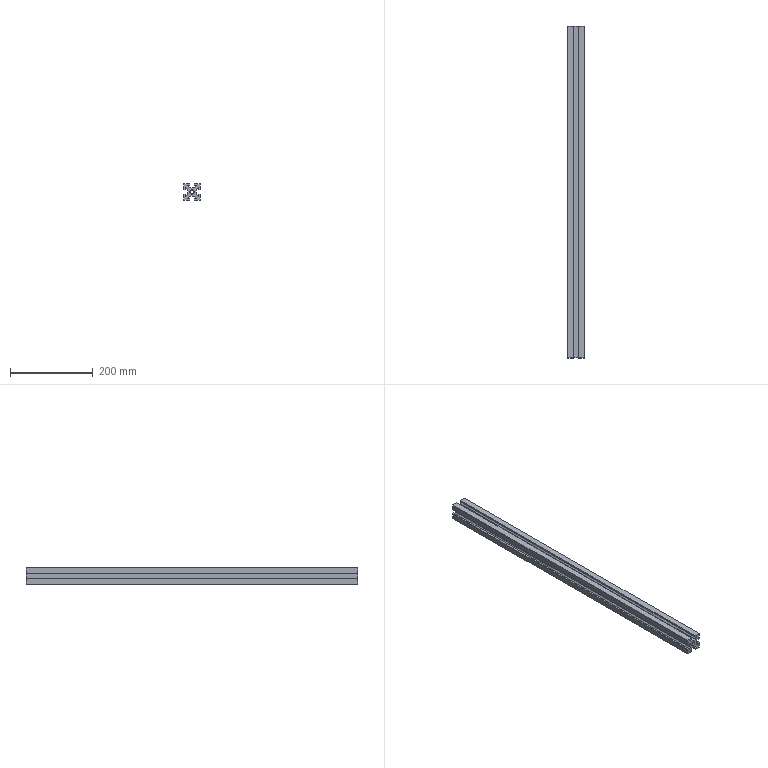Part | SolidWorks | features Extrusion 1 | 1 solid | 40 faces | box 40 x 800 x 40 mm | volume 727286 mm3 | plane 38 | cylinder 2 | commonest cylinder face diameters 10 x2
STEP:
#1=CARTESIAN_POINT('',(0.,800.,-5.));
#2=VERTEX_POINT('',#1);
#3=CARTESIAN_POINT('',(0.,800.,5.));
#4=VERTEX_POINT('',#3);
#5=CARTESIAN_POINT('',(0.,800.,0.));
#6=DIRECTION('',(0.,1.,0.));
#7=DIRECTION('',(0.,0.,1.));
#8=AXIS2_PLACEMENT_3D('',#5,#6,#7);
#9=CIRCLE('',#8,5.);
#10=EDGE_CURVE('',#2,#4,#9,.T.);
#11=ORIENTED_EDGE('',*,*,#10,.T.);
#12=CARTESIAN_POINT('',(0.,0.,5.));
#13=VERTEX_POINT('',#12);
#14=CARTESIAN_POINT('',(0.,800.,5.));
#15=DIRECTION('',(0.,-1.,0.));
#16=VECTOR('',#15,1000.);
#17=LINE('',#14,#16);
#18=EDGE_CURVE('',#4,#13,#17,.T.);
#19=ORIENTED_EDGE('',*,*,#18,.T.);
#20=CARTESIAN_POINT('',(0.,0.,-5.));
#21=VERTEX_POINT('',#20);
#22=CARTESIAN_POINT('',(0.,0.,0.));
#23=DIRECTION('',(0.,1.,0.));
#24=DIRECTION('',(0.,0.,1.));
#25=AXIS2_PLACEMENT_3D('',#22,#23,#24);
#26=CIRCLE('',#25,5.);
#27=EDGE_CURVE('',#21,#13,#26,.T.);
#28=ORIENTED_EDGE('',*,*,#27,.F.);
#29=CARTESIAN_POINT('',(0.,800.,-5.));
#30=DIRECTION('',(0.,-1.,0.));
#31=VECTOR('',#30,1000.);
#32=LINE('',#29,#31);
#33=EDGE_CURVE('',#2,#21,#32,.T.);
#34=ORIENTED_EDGE('',*,*,#33,.F.);
#35=EDGE_LOOP('',(#11,#19,#28,#34));
#36=FACE_OUTER_BOUND('',#35,.T.);
#37=CARTESIAN_POINT('',(0.,800.,0.));
#38=DIRECTION('',(0.,-1.,0.));
#39=DIRECTION('',(0.,0.,-1.));
#40=AXIS2_PLACEMENT_3D('',#37,#38,#39);
#41=CYLINDRICAL_SURFACE('',#40,5.);
#42=ADVANCED_FACE('',(#36),#41,.F.);
#43=CARTESIAN_POINT('',(6.,800.,20.));
#44=VERTEX_POINT('',#43);
#45=CARTESIAN_POINT('',(20.,800.,20.));
#46=VERTEX_POINT('',#45);
#47=CARTESIAN_POINT('',(6.,800.,20.));
#48=DIRECTION('',(1.,0.,0.));
#49=VECTOR('',#48,1000.);
#50=LINE('',#47,#49);
#51=EDGE_CURVE('',#44,#46,#50,.T.);
#52=ORIENTED_EDGE('',*,*,#51,.T.);
#53=CARTESIAN_POINT('',(20.,800.,6.));
#54=VERTEX_POINT('',#53);
#55=CARTESIAN_POINT('',(20.,800.,6.));
#56=DIRECTION('',(0.,0.,-1.));
#57=VECTOR('',#56,1000.);
#58=LINE('',#55,#57);
#59=EDGE_CURVE('',#46,#54,#58,.T.);
#60=ORIENTED_EDGE('',*,*,#59,.T.);
#61=CARTESIAN_POINT('',(16.,800.,6.));
#62=VERTEX_POINT('',#61);
#63=CARTESIAN_POINT('',(16.,800.,6.));
#64=DIRECTION('',(-1.,0.,0.));
#65=VECTOR('',#64,1000.);
#66=LINE('',#63,#65);
#67=EDGE_CURVE('',#54,#62,#66,.T.);
#68=ORIENTED_EDGE('',*,*,#67,.T.);
#69=CARTESIAN_POINT('',(16.,800.,11.757));
#70=VERTEX_POINT('',#69);
#71=CARTESIAN_POINT('',(16.,800.,11.757));
#72=DIRECTION('',(0.,0.,1.));
#73=VECTOR('',#72,1000.);
#74=LINE('',#71,#73);
#75=EDGE_CURVE('',#62,#70,#74,.T.);
#76=ORIENTED_EDGE('',*,*,#75,.T.);
#77=CARTESIAN_POINT('',(10.,800.,5.757));
#78=VERTEX_POINT('',#77);
#79=CARTESIAN_POINT('',(10.,800.,5.757));
#80=DIRECTION('',(-0.7071,0.,-0.7071));
#81=VECTOR('',#80,1000.);
#82=LINE('',#79,#81);
#83=EDGE_CURVE('',#70,#78,#82,.T.);
#84=ORIENTED_EDGE('',*,*,#83,.T.);
#85=CARTESIAN_POINT('',(10.,800.,-5.757));
#86=VERTEX_POINT('',#85);
#87=CARTESIAN_POINT('',(10.,800.,5.757));
#88=DIRECTION('',(0.,0.,-1.));
#89=VECTOR('',#88,1000.);
#90=LINE('',#87,#89);
#91=EDGE_CURVE('',#78,#86,#90,.T.);
#92=ORIENTED_EDGE('',*,*,#91,.T.);
#93=CARTESIAN_POINT('',(16.,800.,-11.757));
#94=VERTEX_POINT('',#93);
#95=CARTESIAN_POINT('',(16.,800.,-11.757));
#96=DIRECTION('',(0.7071,0.,-0.7071));
#97=VECTOR('',#96,1000.);
#98=LINE('',#95,#97);
#99=EDGE_CURVE('',#86,#94,#98,.T.);
#100=ORIENTED_EDGE('',*,*,#99,.T.);
#101=CARTESIAN_POINT('',(16.,800.,-6.));
#102=VERTEX_POINT('',#101);
#103=CARTESIAN_POINT('',(16.,800.,-6.));
#104=DIRECTION('',(0.,0.,1.));
#105=VECTOR('',#104,1000.);
#106=LINE('',#103,#105);
#107=EDGE_CURVE('',#94,#102,#106,.T.);
#108=ORIENTED_EDGE('',*,*,#107,.T.);
#109=CARTESIAN_POINT('',(20.,800.,-6.));
#110=VERTEX_POINT('',#109);
#111=CARTESIAN_POINT('',(20.,800.,-6.));
#112=DIRECTION('',(1.,0.,0.));
#113=VECTOR('',#112,1000.);
#114=LINE('',#111,#113);
#115=EDGE_CURVE('',#102,#110,#114,.T.);
#116=ORIENTED_EDGE('',*,*,#115,.T.);
#117=CARTESIAN_POINT('',(20.,800.,-20.));
#118=VERTEX_POINT('',#117);
#119=CARTESIAN_POINT('',(20.,800.,-20.));
#120=DIRECTION('',(0.,0.,-1.));
#121=VECTOR('',#120,1000.);
#122=LINE('',#119,#121);
#123=EDGE_CURVE('',#110,#118,#122,.T.);
#124=ORIENTED_EDGE('',*,*,#123,.T.);
#125=CARTESIAN_POINT('',(6.,800.,-20.));
#126=VERTEX_POINT('',#125);
#127=CARTESIAN_POINT('',(6.,800.,-20.));
#128=DIRECTION('',(-1.,0.,0.));
#129=VECTOR('',#128,1000.);
#130=LINE('',#127,#129);
#131=EDGE_CURVE('',#118,#126,#130,.T.);
#132=ORIENTED_EDGE('',*,*,#131,.T.);
#133=CARTESIAN_POINT('',(6.,800.,-16.));
#134=VERTEX_POINT('',#133);
#135=CARTESIAN_POINT('',(6.,800.,-16.));
#136=DIRECTION('',(0.,0.,1.));
#137=VECTOR('',#136,1000.);
#138=LINE('',#135,#137);
#139=EDGE_CURVE('',#126,#134,#138,.T.);
#140=ORIENTED_EDGE('',*,*,#139,.T.);
#141=CARTESIAN_POINT('',(11.757,800.,-16.));
#142=VERTEX_POINT('',#141);
#143=CARTESIAN_POINT('',(11.757,800.,-16.));
#144=DIRECTION('',(1.,0.,0.));
#145=VECTOR('',#144,1000.);
#146=LINE('',#143,#145);
#147=EDGE_CURVE('',#134,#142,#146,.T.);
#148=ORIENTED_EDGE('',*,*,#147,.T.);
#149=CARTESIAN_POINT('',(5.757,800.,-10.));
#150=VERTEX_POINT('',#149);
#151=CARTESIAN_POINT('',(5.757,800.,-10.));
#152=DIRECTION('',(-0.7071,0.,0.7071));
#153=VECTOR('',#152,1000.);
#154=LINE('',#151,#153);
#155=EDGE_CURVE('',#142,#150,#154,.T.);
#156=ORIENTED_EDGE('',*,*,#155,.T.);
#157=CARTESIAN_POINT('',(-5.757,800.,-10.));
#158=VERTEX_POINT('',#157);
#159=CARTESIAN_POINT('',(-5.757,800.,-10.));
#160=DIRECTION('',(-1.,0.,0.));
#161=VECTOR('',#160,1000.);
#162=LINE('',#159,#161);
#163=EDGE_CURVE('',#150,#158,#162,.T.);
#164=ORIENTED_EDGE('',*,*,#163,.T.);
#165=CARTESIAN_POINT('',(-11.757,800.,-16.));
#166=VERTEX_POINT('',#165);
#167=CARTESIAN_POINT('',(-11.757,800.,-16.));
#168=DIRECTION('',(-0.7071,0.,-0.7071));
#169=VECTOR('',#168,1000.);
#170=LINE('',#167,#169);
#171=EDGE_CURVE('',#158,#166,#170,.T.);
#172=ORIENTED_EDGE('',*,*,#171,.T.);
#173=CARTESIAN_POINT('',(-6.,800.,-16.));
#174=VERTEX_POINT('',#173);
#175=CARTESIAN_POINT('',(-6.,800.,-16.));
#176=DIRECTION('',(1.,0.,0.));
#177=VECTOR('',#176,1000.);
#178=LINE('',#175,#177);
#179=EDGE_CURVE('',#166,#174,#178,.T.);
#180=ORIENTED_EDGE('',*,*,#179,.T.);
#181=CARTESIAN_POINT('',(-6.,800.,-20.));
#182=VERTEX_POINT('',#181);
#183=CARTESIAN_POINT('',(-6.,800.,-20.));
#184=DIRECTION('',(0.,0.,-1.));
#185=VECTOR('',#184,1000.);
#186=LINE('',#183,#185);
#187=EDGE_CURVE('',#174,#182,#186,.T.);
#188=ORIENTED_EDGE('',*,*,#187,.T.);
#189=CARTESIAN_POINT('',(-20.,800.,-20.));
#190=VERTEX_POINT('',#189);
#191=CARTESIAN_POINT('',(-20.,800.,-20.));
#192=DIRECTION('',(-1.,0.,0.));
#193=VECTOR('',#192,1000.);
#194=LINE('',#191,#193);
#195=EDGE_CURVE('',#182,#190,#194,.T.);
#196=ORIENTED_EDGE('',*,*,#195,.T.);
#197=CARTESIAN_POINT('',(-20.,800.,-6.));
#198=VERTEX_POINT('',#197);
#199=CARTESIAN_POINT('',(-20.,800.,-20.));
#200=DIRECTION('',(0.,0.,1.));
#201=VECTOR('',#200,1000.);
#202=LINE('',#199,#201);
#203=EDGE_CURVE('',#190,#198,#202,.T.);
#204=ORIENTED_EDGE('',*,*,#203,.T.);
#205=CARTESIAN_POINT('',(-16.,800.,-6.));
#206=VERTEX_POINT('',#205);
#207=CARTESIAN_POINT('',(-16.,800.,-6.));
#208=DIRECTION('',(1.,0.,0.));
#209=VECTOR('',#208,1000.);
#210=LINE('',#207,#209);
#211=EDGE_CURVE('',#198,#206,#210,.T.);
#212=ORIENTED_EDGE('',*,*,#211,.T.);
#213=CARTESIAN_POINT('',(-16.,800.,-11.757));
#214=VERTEX_POINT('',#213);
#215=CARTESIAN_POINT('',(-16.,800.,-11.757));
#216=DIRECTION('',(0.,0.,-1.));
#217=VECTOR('',#216,1000.);
#218=LINE('',#215,#217);
#219=EDGE_CURVE('',#206,#214,#218,.T.);
#220=ORIENTED_EDGE('',*,*,#219,.T.);
#221=CARTESIAN_POINT('',(-10.,800.,-5.757));
#222=VERTEX_POINT('',#221);
#223=CARTESIAN_POINT('',(-10.,800.,-5.757));
#224=DIRECTION('',(0.7071,0.,0.7071));
#225=VECTOR('',#224,1000.);
#226=LINE('',#223,#225);
#227=EDGE_CURVE('',#214,#222,#226,.T.);
#228=ORIENTED_EDGE('',*,*,#227,.T.);
#229=CARTESIAN_POINT('',(-10.,800.,5.757));
#230=VERTEX_POINT('',#229);
#231=CARTESIAN_POINT('',(-10.,800.,5.757));
#232=DIRECTION('',(0.,0.,1.));
#233=VECTOR('',#232,1000.);
#234=LINE('',#231,#233);
#235=EDGE_CURVE('',#222,#230,#234,.T.);
#236=ORIENTED_EDGE('',*,*,#235,.T.);
#237=CARTESIAN_POINT('',(-16.,800.,11.757));
#238=VERTEX_POINT('',#237);
#239=CARTESIAN_POINT('',(-16.,800.,11.757));
#240=DIRECTION('',(-0.7071,0.,0.7071));
#241=VECTOR('',#240,1000.);
#242=LINE('',#239,#241);
#243=EDGE_CURVE('',#230,#238,#242,.T.);
#244=ORIENTED_EDGE('',*,*,#243,.T.);
#245=CARTESIAN_POINT('',(-16.,800.,6.));
#246=VERTEX_POINT('',#245);
#247=CARTESIAN_POINT('',(-16.,800.,6.));
#248=DIRECTION('',(0.,0.,-1.));
#249=VECTOR('',#248,1000.);
#250=LINE('',#247,#249);
#251=EDGE_CURVE('',#238,#246,#250,.T.);
#252=ORIENTED_EDGE('',*,*,#251,.T.);
#253=CARTESIAN_POINT('',(-20.,800.,6.));
#254=VERTEX_POINT('',#253);
#255=CARTESIAN_POINT('',(-20.,800.,6.));
#256=DIRECTION('',(-1.,0.,0.));
#257=VECTOR('',#256,1000.);
#258=LINE('',#255,#257);
#259=EDGE_CURVE('',#246,#254,#258,.T.);
#260=ORIENTED_EDGE('',*,*,#259,.T.);
#261=CARTESIAN_POINT('',(-20.,800.,20.));
#262=VERTEX_POINT('',#261);
#263=CARTESIAN_POINT('',(-20.,800.,6.));
#264=DIRECTION('',(0.,0.,1.));
#265=VECTOR('',#264,1000.);
#266=LINE('',#263,#265);
#267=EDGE_CURVE('',#254,#262,#266,.T.);
#268=ORIENTED_EDGE('',*,*,#267,.T.);
#269=CARTESIAN_POINT('',(-6.,800.,20.));
#270=VERTEX_POINT('',#269);
#271=CARTESIAN_POINT('',(-20.,800.,20.));
#272=DIRECTION('',(1.,0.,0.));
#273=VECTOR('',#272,1000.);
#274=LINE('',#271,#273);
#275=EDGE_CURVE('',#262,#270,#274,.T.);
#276=ORIENTED_EDGE('',*,*,#275,.T.);
#277=CARTESIAN_POINT('',(-6.,800.,16.));
#278=VERTEX_POINT('',#277);
#279=CARTESIAN_POINT('',(-6.,800.,16.));
#280=DIRECTION('',(0.,0.,-1.));
#281=VECTOR('',#280,1000.);
#282=LINE('',#279,#281);
#283=EDGE_CURVE('',#270,#278,#282,.T.);
#284=ORIENTED_EDGE('',*,*,#283,.T.);
#285=CARTESIAN_POINT('',(-11.757,800.,16.));
#286=VERTEX_POINT('',#285);
#287=CARTESIAN_POINT('',(-11.757,800.,16.));
#288=DIRECTION('',(-1.,0.,0.));
#289=VECTOR('',#288,1000.);
#290=LINE('',#287,#289);
#291=EDGE_CURVE('',#278,#286,#290,.T.);
#292=ORIENTED_EDGE('',*,*,#291,.T.);
#293=CARTESIAN_POINT('',(-5.757,800.,10.));
#294=VERTEX_POINT('',#293);
#295=CARTESIAN_POINT('',(-5.757,800.,10.));
#296=DIRECTION('',(0.7071,0.,-0.7071));
#297=VECTOR('',#296,1000.);
#298=LINE('',#295,#297);
#299=EDGE_CURVE('',#286,#294,#298,.T.);
#300=ORIENTED_EDGE('',*,*,#299,.T.);
#301=CARTESIAN_POINT('',(5.757,800.,10.));
#302=VERTEX_POINT('',#301);
#303=CARTESIAN_POINT('',(-5.757,800.,10.));
#304=DIRECTION('',(1.,0.,0.));
#305=VECTOR('',#304,1000.);
#306=LINE('',#303,#305);
#307=EDGE_CURVE('',#294,#302,#306,.T.);
#308=ORIENTED_EDGE('',*,*,#307,.T.);
#309=CARTESIAN_POINT('',(11.757,800.,16.));
#310=VERTEX_POINT('',#309);
#311=CARTESIAN_POINT('',(11.757,800.,16.));
#312=DIRECTION('',(0.7071,0.,0.7071));
#313=VECTOR('',#312,1000.);
#314=LINE('',#311,#313);
#315=EDGE_CURVE('',#302,#310,#314,.T.);
#316=ORIENTED_EDGE('',*,*,#315,.T.);
#317=CARTESIAN_POINT('',(6.,800.,16.));
#318=VERTEX_POINT('',#317);
#319=CARTESIAN_POINT('',(6.,800.,16.));
#320=DIRECTION('',(-1.,0.,0.));
#321=VECTOR('',#320,1000.);
#322=LINE('',#319,#321);
#323=EDGE_CURVE('',#310,#318,#322,.T.);
#324=ORIENTED_EDGE('',*,*,#323,.T.);
#325=CARTESIAN_POINT('',(6.,800.,20.));
#326=DIRECTION('',(0.,0.,1.));
#327=VECTOR('',#326,1000.);
#328=LINE('',#325,#327);
#329=EDGE_CURVE('',#318,#44,#328,.T.);
#330=ORIENTED_EDGE('',*,*,#329,.T.);
#331=EDGE_LOOP('',(#52,#60,#68,#76,#84,#92,#100,#108,#116,#124,#132,#140,#148,#156,#164,#172,#180,#188,#196,#204,#212,#220,#228,#236,#244,#252,#260,#268,#276,#284,#292,#300,#308,#316,#324,#330));
#332=FACE_OUTER_BOUND('',#331,.T.);
#333=ORIENTED_EDGE('',*,*,#10,.F.);
#334=CARTESIAN_POINT('',(0.,800.,0.));
#335=DIRECTION('',(0.,1.,0.));
#336=DIRECTION('',(0.,0.,1.));
#337=AXIS2_PLACEMENT_3D('',#334,#335,#336);
#338=CIRCLE('',#337,5.);
#339=EDGE_CURVE('',#4,#2,#338,.T.);
#340=ORIENTED_EDGE('',*,*,#339,.F.);
#341=EDGE_LOOP('',(#333,#340));
#342=FACE_BOUND('',#341,.T.);
#343=CARTESIAN_POINT('',(0.,800.,0.));
#344=DIRECTION('',(0.,-1.,0.));
#345=DIRECTION('',(0.,0.,-1.));
#346=AXIS2_PLACEMENT_3D('',#343,#344,#345);
#347=PLANE('',#346);
#348=ADVANCED_FACE('',(#332,#342),#347,.F.);
#349=CARTESIAN_POINT('',(6.,0.,20.));
#350=VERTEX_POINT('',#349);
#351=CARTESIAN_POINT('',(20.,0.,20.));
#352=VERTEX_POINT('',#351);
#353=CARTESIAN_POINT('',(6.,0.,20.));
#354=DIRECTION('',(1.,0.,0.));
#355=VECTOR('',#354,1000.);
#356=LINE('',#353,#355);
#357=EDGE_CURVE('',#350,#352,#356,.T.);
#358=ORIENTED_EDGE('',*,*,#357,.F.);
#359=CARTESIAN_POINT('',(6.,0.,16.));
#360=VERTEX_POINT('',#359);
#361=CARTESIAN_POINT('',(6.,0.,20.));
#362=DIRECTION('',(0.,0.,1.));
#363=VECTOR('',#362,1000.);
#364=LINE('',#361,#363);
#365=EDGE_CURVE('',#360,#350,#364,.T.);
#366=ORIENTED_EDGE('',*,*,#365,.F.);
#367=CARTESIAN_POINT('',(11.757,0.,16.));
#368=VERTEX_POINT('',#367);
#369=CARTESIAN_POINT('',(6.,0.,16.));
#370=DIRECTION('',(-1.,0.,0.));
#371=VECTOR('',#370,1000.);
#372=LINE('',#369,#371);
#373=EDGE_CURVE('',#368,#360,#372,.T.);
#374=ORIENTED_EDGE('',*,*,#373,.F.);
#375=CARTESIAN_POINT('',(5.757,0.,10.));
#376=VERTEX_POINT('',#375);
#377=CARTESIAN_POINT('',(11.757,0.,16.));
#378=DIRECTION('',(0.7071,0.,0.7071));
#379=VECTOR('',#378,1000.);
#380=LINE('',#377,#379);
#381=EDGE_CURVE('',#376,#368,#380,.T.);
#382=ORIENTED_EDGE('',*,*,#381,.F.);
#383=CARTESIAN_POINT('',(-5.757,0.,10.));
#384=VERTEX_POINT('',#383);
#385=CARTESIAN_POINT('',(-5.757,0.,10.));
#386=DIRECTION('',(1.,0.,0.));
#387=VECTOR('',#386,1000.);
#388=LINE('',#385,#387);
#389=EDGE_CURVE('',#384,#376,#388,.T.);
#390=ORIENTED_EDGE('',*,*,#389,.F.);
#391=CARTESIAN_POINT('',(-11.757,0.,16.));
#392=VERTEX_POINT('',#391);
#393=CARTESIAN_POINT('',(-5.757,0.,10.));
#394=DIRECTION('',(0.7071,0.,-0.7071));
#395=VECTOR('',#394,1000.);
#396=LINE('',#393,#395);
#397=EDGE_CURVE('',#392,#384,#396,.T.);
#398=ORIENTED_EDGE('',*,*,#397,.F.);
#399=CARTESIAN_POINT('',(-6.,0.,16.));
#400=VERTEX_POINT('',#399);
#401=CARTESIAN_POINT('',(-11.757,0.,16.));
#402=DIRECTION('',(-1.,0.,0.));
#403=VECTOR('',#402,1000.);
#404=LINE('',#401,#403);
#405=EDGE_CURVE('',#400,#392,#404,.T.);
#406=ORIENTED_EDGE('',*,*,#405,.F.);
#407=CARTESIAN_POINT('',(-6.,0.,20.));
#408=VERTEX_POINT('',#407);
#409=CARTESIAN_POINT('',(-6.,0.,16.));
#410=DIRECTION('',(0.,0.,-1.));
#411=VECTOR('',#410,1000.);
#412=LINE('',#409,#411);
#413=EDGE_CURVE('',#408,#400,#412,.T.);
#414=ORIENTED_EDGE('',*,*,#413,.F.);
#415=CARTESIAN_POINT('',(-20.,0.,20.));
#416=VERTEX_POINT('',#415);
#417=CARTESIAN_POINT('',(-20.,0.,20.));
#418=DIRECTION('',(1.,0.,0.));
#419=VECTOR('',#418,1000.);
#420=LINE('',#417,#419);
#421=EDGE_CURVE('',#416,#408,#420,.T.);
#422=ORIENTED_EDGE('',*,*,#421,.F.);
#423=CARTESIAN_POINT('',(-20.,0.,6.));
#424=VERTEX_POINT('',#423);
#425=CARTESIAN_POINT('',(-20.,0.,6.));
#426=DIRECTION('',(0.,0.,1.));
#427=VECTOR('',#426,1000.);
#428=LINE('',#425,#427);
#429=EDGE_CURVE('',#424,#416,#428,.T.);
#430=ORIENTED_EDGE('',*,*,#429,.F.);
#431=CARTESIAN_POINT('',(-16.,0.,6.));
#432=VERTEX_POINT('',#431);
#433=CARTESIAN_POINT('',(-20.,0.,6.));
#434=DIRECTION('',(-1.,0.,0.));
#435=VECTOR('',#434,1000.);
#436=LINE('',#433,#435);
#437=EDGE_CURVE('',#432,#424,#436,.T.);
#438=ORIENTED_EDGE('',*,*,#437,.F.);
#439=CARTESIAN_POINT('',(-16.,0.,11.757));
#440=VERTEX_POINT('',#439);
#441=CARTESIAN_POINT('',(-16.,0.,6.));
#442=DIRECTION('',(0.,0.,-1.));
#443=VECTOR('',#442,1000.);
#444=LINE('',#441,#443);
#445=EDGE_CURVE('',#440,#432,#444,.T.);
#446=ORIENTED_EDGE('',*,*,#445,.F.);
#447=CARTESIAN_POINT('',(-10.,0.,5.757));
#448=VERTEX_POINT('',#447);
#449=CARTESIAN_POINT('',(-16.,0.,11.757));
#450=DIRECTION('',(-0.7071,0.,0.7071));
#451=VECTOR('',#450,1000.);
#452=LINE('',#449,#451);
#453=EDGE_CURVE('',#448,#440,#452,.T.);
#454=ORIENTED_EDGE('',*,*,#453,.F.);
#455=CARTESIAN_POINT('',(-10.,0.,-5.757));
#456=VERTEX_POINT('',#455);
#457=CARTESIAN_POINT('',(-10.,0.,5.757));
#458=DIRECTION('',(0.,0.,1.));
#459=VECTOR('',#458,1000.);
#460=LINE('',#457,#459);
#461=EDGE_CURVE('',#456,#448,#460,.T.);
#462=ORIENTED_EDGE('',*,*,#461,.F.);
#463=CARTESIAN_POINT('',(-16.,0.,-11.757));
#464=VERTEX_POINT('',#463);
#465=CARTESIAN_POINT('',(-10.,0.,-5.757));
#466=DIRECTION('',(0.7071,0.,0.7071));
#467=VECTOR('',#466,1000.);
#468=LINE('',#465,#467);
#469=EDGE_CURVE('',#464,#456,#468,.T.);
#470=ORIENTED_EDGE('',*,*,#469,.F.);
#471=CARTESIAN_POINT('',(-16.,0.,-6.));
#472=VERTEX_POINT('',#471);
#473=CARTESIAN_POINT('',(-16.,0.,-11.757));
#474=DIRECTION('',(0.,0.,-1.));
#475=VECTOR('',#474,1000.);
#476=LINE('',#473,#475);
#477=EDGE_CURVE('',#472,#464,#476,.T.);
#478=ORIENTED_EDGE('',*,*,#477,.F.);
#479=CARTESIAN_POINT('',(-20.,0.,-6.));
#480=VERTEX_POINT('',#479);
#481=CARTESIAN_POINT('',(-16.,0.,-6.));
#482=DIRECTION('',(1.,0.,0.));
#483=VECTOR('',#482,1000.);
#484=LINE('',#481,#483);
#485=EDGE_CURVE('',#480,#472,#484,.T.);
#486=ORIENTED_EDGE('',*,*,#485,.F.);
#487=CARTESIAN_POINT('',(-20.,0.,-20.));
#488=VERTEX_POINT('',#487);
#489=CARTESIAN_POINT('',(-20.,0.,-20.));
#490=DIRECTION('',(0.,0.,1.));
#491=VECTOR('',#490,1000.);
#492=LINE('',#489,#491);
#493=EDGE_CURVE('',#488,#480,#492,.T.);
#494=ORIENTED_EDGE('',*,*,#493,.F.);
#495=CARTESIAN_POINT('',(-6.,0.,-20.));
#496=VERTEX_POINT('',#495);
#497=CARTESIAN_POINT('',(-20.,0.,-20.));
#498=DIRECTION('',(-1.,0.,0.));
#499=VECTOR('',#498,1000.);
#500=LINE('',#497,#499);
#501=EDGE_CURVE('',#496,#488,#500,.T.);
#502=ORIENTED_EDGE('',*,*,#501,.F.);
#503=CARTESIAN_POINT('',(-6.,0.,-16.));
#504=VERTEX_POINT('',#503);
#505=CARTESIAN_POINT('',(-6.,0.,-20.));
#506=DIRECTION('',(0.,0.,-1.));
#507=VECTOR('',#506,1000.);
#508=LINE('',#505,#507);
#509=EDGE_CURVE('',#504,#496,#508,.T.);
#510=ORIENTED_EDGE('',*,*,#509,.F.);
#511=CARTESIAN_POINT('',(-11.757,0.,-16.));
#512=VERTEX_POINT('',#511);
#513=CARTESIAN_POINT('',(-6.,0.,-16.));
#514=DIRECTION('',(1.,0.,0.));
#515=VECTOR('',#514,1000.);
#516=LINE('',#513,#515);
#517=EDGE_CURVE('',#512,#504,#516,.T.);
#518=ORIENTED_EDGE('',*,*,#517,.F.);
#519=CARTESIAN_POINT('',(-5.757,0.,-10.));
#520=VERTEX_POINT('',#519);
#521=CARTESIAN_POINT('',(-11.757,0.,-16.));
#522=DIRECTION('',(-0.7071,0.,-0.7071));
#523=VECTOR('',#522,1000.);
#524=LINE('',#521,#523);
#525=EDGE_CURVE('',#520,#512,#524,.T.);
#526=ORIENTED_EDGE('',*,*,#525,.F.);
#527=CARTESIAN_POINT('',(5.757,0.,-10.));
#528=VERTEX_POINT('',#527);
#529=CARTESIAN_POINT('',(-5.757,0.,-10.));
#530=DIRECTION('',(-1.,0.,0.));
#531=VECTOR('',#530,1000.);
#532=LINE('',#529,#531);
#533=EDGE_CURVE('',#528,#520,#532,.T.);
#534=ORIENTED_EDGE('',*,*,#533,.F.);
#535=CARTESIAN_POINT('',(11.757,0.,-16.));
#536=VERTEX_POINT('',#535);
#537=CARTESIAN_POINT('',(5.757,0.,-10.));
#538=DIRECTION('',(-0.7071,0.,0.7071));
#539=VECTOR('',#538,1000.);
#540=LINE('',#537,#539);
#541=EDGE_CURVE('',#536,#528,#540,.T.);
#542=ORIENTED_EDGE('',*,*,#541,.F.);
#543=CARTESIAN_POINT('',(6.,0.,-16.));
#544=VERTEX_POINT('',#543);
#545=CARTESIAN_POINT('',(11.757,0.,-16.));
#546=DIRECTION('',(1.,0.,0.));
#547=VECTOR('',#546,1000.);
#548=LINE('',#545,#547);
#549=EDGE_CURVE('',#544,#536,#548,.T.);
#550=ORIENTED_EDGE('',*,*,#549,.F.);
#551=CARTESIAN_POINT('',(6.,0.,-20.));
#552=VERTEX_POINT('',#551);
#553=CARTESIAN_POINT('',(6.,0.,-16.));
#554=DIRECTION('',(0.,0.,1.));
#555=VECTOR('',#554,1000.);
#556=LINE('',#553,#555);
#557=EDGE_CURVE('',#552,#544,#556,.T.);
#558=ORIENTED_EDGE('',*,*,#557,.F.);
#559=CARTESIAN_POINT('',(20.,0.,-20.));
#560=VERTEX_POINT('',#559);
#561=CARTESIAN_POINT('',(6.,0.,-20.));
#562=DIRECTION('',(-1.,0.,0.));
#563=VECTOR('',#562,1000.);
#564=LINE('',#561,#563);
#565=EDGE_CURVE('',#560,#552,#564,.T.);
#566=ORIENTED_EDGE('',*,*,#565,.F.);
#567=CARTESIAN_POINT('',(20.,0.,-6.));
#568=VERTEX_POINT('',#567);
#569=CARTESIAN_POINT('',(20.,0.,-20.));
#570=DIRECTION('',(0.,0.,-1.));
#571=VECTOR('',#570,1000.);
#572=LINE('',#569,#571);
#573=EDGE_CURVE('',#568,#560,#572,.T.);
#574=ORIENTED_EDGE('',*,*,#573,.F.);
#575=CARTESIAN_POINT('',(16.,0.,-6.));
#576=VERTEX_POINT('',#575);
#577=CARTESIAN_POINT('',(20.,0.,-6.));
#578=DIRECTION('',(1.,0.,0.));
#579=VECTOR('',#578,1000.);
#580=LINE('',#577,#579);
#581=EDGE_CURVE('',#576,#568,#580,.T.);
#582=ORIENTED_EDGE('',*,*,#581,.F.);
#583=CARTESIAN_POINT('',(16.,0.,-11.757));
#584=VERTEX_POINT('',#583);
#585=CARTESIAN_POINT('',(16.,0.,-6.));
#586=DIRECTION('',(0.,0.,1.));
#587=VECTOR('',#586,1000.);
#588=LINE('',#585,#587);
#589=EDGE_CURVE('',#584,#576,#588,.T.);
#590=ORIENTED_EDGE('',*,*,#589,.F.);
#591=CARTESIAN_POINT('',(10.,0.,-5.757));
#592=VERTEX_POINT('',#591);
#593=CARTESIAN_POINT('',(16.,0.,-11.757));
#594=DIRECTION('',(0.7071,0.,-0.7071));
#595=VECTOR('',#594,1000.);
#596=LINE('',#593,#595);
#597=EDGE_CURVE('',#592,#584,#596,.T.);
#598=ORIENTED_EDGE('',*,*,#597,.F.);
#599=CARTESIAN_POINT('',(10.,0.,5.757));
#600=VERTEX_POINT('',#599);
#601=CARTESIAN_POINT('',(10.,0.,5.757));
#602=DIRECTION('',(0.,0.,-1.));
#603=VECTOR('',#602,1000.);
#604=LINE('',#601,#603);
#605=EDGE_CURVE('',#600,#592,#604,.T.);
#606=ORIENTED_EDGE('',*,*,#605,.F.);
#607=CARTESIAN_POINT('',(16.,0.,11.757));
#608=VERTEX_POINT('',#607);
#609=CARTESIAN_POINT('',(10.,0.,5.757));
#610=DIRECTION('',(-0.7071,0.,-0.7071));
#611=VECTOR('',#610,1000.);
#612=LINE('',#609,#611);
#613=EDGE_CURVE('',#608,#600,#612,.T.);
#614=ORIENTED_EDGE('',*,*,#613,.F.);
#615=CARTESIAN_POINT('',(16.,0.,6.));
#616=VERTEX_POINT('',#615);
#617=CARTESIAN_POINT('',(16.,0.,11.757));
#618=DIRECTION('',(0.,0.,1.));
#619=VECTOR('',#618,1000.);
#620=LINE('',#617,#619);
#621=EDGE_CURVE('',#616,#608,#620,.T.);
#622=ORIENTED_EDGE('',*,*,#621,.F.);
#623=CARTESIAN_POINT('',(20.,0.,6.));
#624=VERTEX_POINT('',#623);
#625=CARTESIAN_POINT('',(16.,0.,6.));
#626=DIRECTION('',(-1.,0.,0.));
#627=VECTOR('',#626,1000.);
#628=LINE('',#625,#627);
#629=EDGE_CURVE('',#624,#616,#628,.T.);
#630=ORIENTED_EDGE('',*,*,#629,.F.);
#631=CARTESIAN_POINT('',(20.,0.,6.));
#632=DIRECTION('',(0.,0.,-1.));
#633=VECTOR('',#632,1000.);
#634=LINE('',#631,#633);
#635=EDGE_CURVE('',#352,#624,#634,.T.);
#636=ORIENTED_EDGE('',*,*,#635,.F.);
#637=EDGE_LOOP('',(#358,#366,#374,#382,#390,#398,#406,#414,#422,#430,#438,#446,#454,#462,#470,#478,#486,#494,#502,#510,#518,#526,#534,#542,#550,#558,#566,#574,#582,#590,#598,#606,#614,#622,#630,#636));
#638=FACE_OUTER_BOUND('',#637,.T.);
#639=ORIENTED_EDGE('',*,*,#27,.T.);
#640=CARTESIAN_POINT('',(0.,0.,0.));
#641=DIRECTION('',(0.,1.,0.));
#642=DIRECTION('',(0.,0.,1.));
#643=AXIS2_PLACEMENT_3D('',#640,#641,#642);
#644=CIRCLE('',#643,5.);
#645=EDGE_CURVE('',#13,#21,#644,.T.);
#646=ORIENTED_EDGE('',*,*,#645,.T.);
#647=EDGE_LOOP('',(#639,#646));
#648=FACE_BOUND('',#647,.T.);
#649=CARTESIAN_POINT('',(0.,0.,0.));
#650=DIRECTION('',(0.,-1.,0.));
#651=DIRECTION('',(0.,0.,-1.));
#652=AXIS2_PLACEMENT_3D('',#649,#650,#651);
#653=PLANE('',#652);
#654=ADVANCED_FACE('',(#638,#648),#653,.T.);
#655=ORIENTED_EDGE('',*,*,#357,.T.);
#656=CARTESIAN_POINT('',(20.,800.,20.));
#657=DIRECTION('',(0.,-1.,0.));
#658=VECTOR('',#657,1000.);
#659=LINE('',#656,#658);
#660=EDGE_CURVE('',#46,#352,#659,.T.);
#661=ORIENTED_EDGE('',*,*,#660,.F.);
#662=ORIENTED_EDGE('',*,*,#51,.F.);
#663=CARTESIAN_POINT('',(6.,800.,20.));
#664=DIRECTION('',(0.,-1.,0.));
#665=VECTOR('',#664,1000.);
#666=LINE('',#663,#665);
#667=EDGE_CURVE('',#44,#350,#666,.T.);
#668=ORIENTED_EDGE('',*,*,#667,.T.);
#669=EDGE_LOOP('',(#655,#661,#662,#668));
#670=FACE_OUTER_BOUND('',#669,.T.);
#671=CARTESIAN_POINT('',(6.,800.,20.));
#672=DIRECTION('',(0.,0.,-1.));
#673=DIRECTION('',(-1.,0.,0.));
#674=AXIS2_PLACEMENT_3D('',#671,#672,#673);
#675=PLANE('',#674);
#676=ADVANCED_FACE('',(#670),#675,.F.);
#677=ORIENTED_EDGE('',*,*,#635,.T.);
#678=CARTESIAN_POINT('',(20.,800.,6.));
#679=DIRECTION('',(0.,-1.,0.));
#680=VECTOR('',#679,1000.);
#681=LINE('',#678,#680);
#682=EDGE_CURVE('',#54,#624,#681,.T.);
#683=ORIENTED_EDGE('',*,*,#682,.F.);
#684=ORIENTED_EDGE('',*,*,#59,.F.);
#685=ORIENTED_EDGE('',*,*,#660,.T.);
#686=EDGE_LOOP('',(#677,#683,#684,#685));
#687=FACE_OUTER_BOUND('',#686,.T.);
#688=CARTESIAN_POINT('',(20.,800.,6.));
#689=DIRECTION('',(-1.,0.,0.));
#690=DIRECTION('',(0.,0.,1.));
#691=AXIS2_PLACEMENT_3D('',#688,#689,#690);
#692=PLANE('',#691);
#693=ADVANCED_FACE('',(#687),#692,.F.);
#694=ORIENTED_EDGE('',*,*,#629,.T.);
#695=CARTESIAN_POINT('',(16.,800.,6.));
#696=DIRECTION('',(0.,-1.,0.));
#697=VECTOR('',#696,1000.);
#698=LINE('',#695,#697);
#699=EDGE_CURVE('',#62,#616,#698,.T.);
#700=ORIENTED_EDGE('',*,*,#699,.F.);
#701=ORIENTED_EDGE('',*,*,#67,.F.);
#702=ORIENTED_EDGE('',*,*,#682,.T.);
#703=EDGE_LOOP('',(#694,#700,#701,#702));
#704=FACE_OUTER_BOUND('',#703,.T.);
#705=CARTESIAN_POINT('',(16.,800.,6.));
#706=DIRECTION('',(0.,0.,1.));
#707=DIRECTION('',(1.,0.,0.));
#708=AXIS2_PLACEMENT_3D('',#705,#706,#707);
#709=PLANE('',#708);
#710=ADVANCED_FACE('',(#704),#709,.F.);
#711=ORIENTED_EDGE('',*,*,#621,.T.);
#712=CARTESIAN_POINT('',(16.,800.,11.757));
#713=DIRECTION('',(0.,-1.,0.));
#714=VECTOR('',#713,1000.);
#715=LINE('',#712,#714);
#716=EDGE_CURVE('',#70,#608,#715,.T.);
#717=ORIENTED_EDGE('',*,*,#716,.F.);
#718=ORIENTED_EDGE('',*,*,#75,.F.);
#719=ORIENTED_EDGE('',*,*,#699,.T.);
#720=EDGE_LOOP('',(#711,#717,#718,#719));
#721=FACE_OUTER_BOUND('',#720,.T.);
#722=CARTESIAN_POINT('',(16.,800.,11.757));
#723=DIRECTION('',(1.,0.,0.));
#724=DIRECTION('',(0.,0.,-1.));
#725=AXIS2_PLACEMENT_3D('',#722,#723,#724);
#726=PLANE('',#725);
#727=ADVANCED_FACE('',(#721),#726,.F.);
#728=ORIENTED_EDGE('',*,*,#613,.T.);
#729=CARTESIAN_POINT('',(10.,800.,5.757));
#730=DIRECTION('',(0.,-1.,0.));
#731=VECTOR('',#730,1000.);
#732=LINE('',#729,#731);
#733=EDGE_CURVE('',#78,#600,#732,.T.);
#734=ORIENTED_EDGE('',*,*,#733,.F.);
#735=ORIENTED_EDGE('',*,*,#83,.F.);
#736=ORIENTED_EDGE('',*,*,#716,.T.);
#737=EDGE_LOOP('',(#728,#734,#735,#736));
#738=FACE_OUTER_BOUND('',#737,.T.);
#739=CARTESIAN_POINT('',(10.,800.,5.757));
#740=DIRECTION('',(-0.7071,0.,0.7071));
#741=DIRECTION('',(0.7071,0.,0.7071));
#742=AXIS2_PLACEMENT_3D('',#739,#740,#741);
#743=PLANE('',#742);
#744=ADVANCED_FACE('',(#738),#743,.F.);
#745=ORIENTED_EDGE('',*,*,#605,.T.);
#746=CARTESIAN_POINT('',(10.,800.,-5.757));
#747=DIRECTION('',(0.,-1.,0.));
#748=VECTOR('',#747,1000.);
#749=LINE('',#746,#748);
#750=EDGE_CURVE('',#86,#592,#749,.T.);
#751=ORIENTED_EDGE('',*,*,#750,.F.);
#752=ORIENTED_EDGE('',*,*,#91,.F.);
#753=ORIENTED_EDGE('',*,*,#733,.T.);
#754=EDGE_LOOP('',(#745,#751,#752,#753));
#755=FACE_OUTER_BOUND('',#754,.T.);
#756=CARTESIAN_POINT('',(10.,800.,5.757));
#757=DIRECTION('',(-1.,0.,0.));
#758=DIRECTION('',(0.,0.,1.));
#759=AXIS2_PLACEMENT_3D('',#756,#757,#758);
#760=PLANE('',#759);
#761=ADVANCED_FACE('',(#755),#760,.F.);
#762=ORIENTED_EDGE('',*,*,#597,.T.);
#763=CARTESIAN_POINT('',(16.,800.,-11.757));
#764=DIRECTION('',(0.,-1.,0.));
#765=VECTOR('',#764,1000.);
#766=LINE('',#763,#765);
#767=EDGE_CURVE('',#94,#584,#766,.T.);
#768=ORIENTED_EDGE('',*,*,#767,.F.);
#769=ORIENTED_EDGE('',*,*,#99,.F.);
#770=ORIENTED_EDGE('',*,*,#750,.T.);
#771=EDGE_LOOP('',(#762,#768,#769,#770));
#772=FACE_OUTER_BOUND('',#771,.T.);
#773=CARTESIAN_POINT('',(16.,800.,-11.757));
#774=DIRECTION('',(-0.7071,0.,-0.7071));
#775=DIRECTION('',(-0.7071,0.,0.7071));
#776=AXIS2_PLACEMENT_3D('',#773,#774,#775);
#777=PLANE('',#776);
#778=ADVANCED_FACE('',(#772),#777,.F.);
#779=ORIENTED_EDGE('',*,*,#589,.T.);
#780=CARTESIAN_POINT('',(16.,800.,-6.));
#781=DIRECTION('',(0.,-1.,0.));
#782=VECTOR('',#781,1000.);
#783=LINE('',#780,#782);
#784=EDGE_CURVE('',#102,#576,#783,.T.);
#785=ORIENTED_EDGE('',*,*,#784,.F.);
#786=ORIENTED_EDGE('',*,*,#107,.F.);
#787=ORIENTED_EDGE('',*,*,#767,.T.);
#788=EDGE_LOOP('',(#779,#785,#786,#787));
#789=FACE_OUTER_BOUND('',#788,.T.);
#790=CARTESIAN_POINT('',(16.,800.,-6.));
#791=DIRECTION('',(1.,0.,0.));
#792=DIRECTION('',(0.,0.,-1.));
#793=AXIS2_PLACEMENT_3D('',#790,#791,#792);
#794=PLANE('',#793);
#795=ADVANCED_FACE('',(#789),#794,.F.);
#796=ORIENTED_EDGE('',*,*,#581,.T.);
#797=CARTESIAN_POINT('',(20.,800.,-6.));
#798=DIRECTION('',(0.,-1.,0.));
#799=VECTOR('',#798,1000.);
#800=LINE('',#797,#799);
#801=EDGE_CURVE('',#110,#568,#800,.T.);
#802=ORIENTED_EDGE('',*,*,#801,.F.);
#803=ORIENTED_EDGE('',*,*,#115,.F.);
#804=ORIENTED_EDGE('',*,*,#784,.T.);
#805=EDGE_LOOP('',(#796,#802,#803,#804));
#806=FACE_OUTER_BOUND('',#805,.T.);
#807=CARTESIAN_POINT('',(20.,800.,-6.));
#808=DIRECTION('',(0.,0.,-1.));
#809=DIRECTION('',(-1.,0.,0.));
#810=AXIS2_PLACEMENT_3D('',#807,#808,#809);
#811=PLANE('',#810);
#812=ADVANCED_FACE('',(#806),#811,.F.);
#813=ORIENTED_EDGE('',*,*,#573,.T.);
#814=CARTESIAN_POINT('',(20.,800.,-20.));
#815=DIRECTION('',(0.,-1.,0.));
#816=VECTOR('',#815,1000.);
#817=LINE('',#814,#816);
#818=EDGE_CURVE('',#118,#560,#817,.T.);
#819=ORIENTED_EDGE('',*,*,#818,.F.);
#820=ORIENTED_EDGE('',*,*,#123,.F.);
#821=ORIENTED_EDGE('',*,*,#801,.T.);
#822=EDGE_LOOP('',(#813,#819,#820,#821));
#823=FACE_OUTER_BOUND('',#822,.T.);
#824=CARTESIAN_POINT('',(20.,800.,-20.));
#825=DIRECTION('',(-1.,0.,0.));
#826=DIRECTION('',(0.,0.,1.));
#827=AXIS2_PLACEMENT_3D('',#824,#825,#826);
#828=PLANE('',#827);
#829=ADVANCED_FACE('',(#823),#828,.F.);
#830=ORIENTED_EDGE('',*,*,#565,.T.);
#831=CARTESIAN_POINT('',(6.,800.,-20.));
#832=DIRECTION('',(0.,-1.,0.));
#833=VECTOR('',#832,1000.);
#834=LINE('',#831,#833);
#835=EDGE_CURVE('',#126,#552,#834,.T.);
#836=ORIENTED_EDGE('',*,*,#835,.F.);
#837=ORIENTED_EDGE('',*,*,#131,.F.);
#838=ORIENTED_EDGE('',*,*,#818,.T.);
#839=EDGE_LOOP('',(#830,#836,#837,#838));
#840=FACE_OUTER_BOUND('',#839,.T.);
#841=CARTESIAN_POINT('',(6.,800.,-20.));
#842=DIRECTION('',(0.,0.,1.));
#843=DIRECTION('',(1.,0.,0.));
#844=AXIS2_PLACEMENT_3D('',#841,#842,#843);
#845=PLANE('',#844);
#846=ADVANCED_FACE('',(#840),#845,.F.);
#847=ORIENTED_EDGE('',*,*,#557,.T.);
#848=CARTESIAN_POINT('',(6.,800.,-16.));
#849=DIRECTION('',(0.,-1.,0.));
#850=VECTOR('',#849,1000.);
#851=LINE('',#848,#850);
#852=EDGE_CURVE('',#134,#544,#851,.T.);
#853=ORIENTED_EDGE('',*,*,#852,.F.);
#854=ORIENTED_EDGE('',*,*,#139,.F.);
#855=ORIENTED_EDGE('',*,*,#835,.T.);
#856=EDGE_LOOP('',(#847,#853,#854,#855));
#857=FACE_OUTER_BOUND('',#856,.T.);
#858=CARTESIAN_POINT('',(6.,800.,-16.));
#859=DIRECTION('',(1.,0.,0.));
#860=DIRECTION('',(0.,0.,-1.));
#861=AXIS2_PLACEMENT_3D('',#858,#859,#860);
#862=PLANE('',#861);
#863=ADVANCED_FACE('',(#857),#862,.F.);
#864=ORIENTED_EDGE('',*,*,#549,.T.);
#865=CARTESIAN_POINT('',(11.757,800.,-16.));
#866=DIRECTION('',(0.,-1.,0.));
#867=VECTOR('',#866,1000.);
#868=LINE('',#865,#867);
#869=EDGE_CURVE('',#142,#536,#868,.T.);
#870=ORIENTED_EDGE('',*,*,#869,.F.);
#871=ORIENTED_EDGE('',*,*,#147,.F.);
#872=ORIENTED_EDGE('',*,*,#852,.T.);
#873=EDGE_LOOP('',(#864,#870,#871,#872));
#874=FACE_OUTER_BOUND('',#873,.T.);
#875=CARTESIAN_POINT('',(11.757,800.,-16.));
#876=DIRECTION('',(0.,0.,-1.));
#877=DIRECTION('',(-1.,0.,0.));
#878=AXIS2_PLACEMENT_3D('',#875,#876,#877);
#879=PLANE('',#878);
#880=ADVANCED_FACE('',(#874),#879,.F.);
#881=ORIENTED_EDGE('',*,*,#541,.T.);
#882=CARTESIAN_POINT('',(5.757,800.,-10.));
#883=DIRECTION('',(0.,-1.,0.));
#884=VECTOR('',#883,1000.);
#885=LINE('',#882,#884);
#886=EDGE_CURVE('',#150,#528,#885,.T.);
#887=ORIENTED_EDGE('',*,*,#886,.F.);
#888=ORIENTED_EDGE('',*,*,#155,.F.);
#889=ORIENTED_EDGE('',*,*,#869,.T.);
#890=EDGE_LOOP('',(#881,#887,#888,#889));
#891=FACE_OUTER_BOUND('',#890,.T.);
#892=CARTESIAN_POINT('',(5.757,800.,-10.));
#893=DIRECTION('',(0.7071,0.,0.7071));
#894=DIRECTION('',(0.7071,0.,-0.7071));
#895=AXIS2_PLACEMENT_3D('',#892,#893,#894);
#896=PLANE('',#895);
#897=ADVANCED_FACE('',(#891),#896,.F.);
#898=ORIENTED_EDGE('',*,*,#533,.T.);
#899=CARTESIAN_POINT('',(-5.757,800.,-10.));
#900=DIRECTION('',(0.,-1.,0.));
#901=VECTOR('',#900,1000.);
#902=LINE('',#899,#901);
#903=EDGE_CURVE('',#158,#520,#902,.T.);
#904=ORIENTED_EDGE('',*,*,#903,.F.);
#905=ORIENTED_EDGE('',*,*,#163,.F.);
#906=ORIENTED_EDGE('',*,*,#886,.T.);
#907=EDGE_LOOP('',(#898,#904,#905,#906));
#908=FACE_OUTER_BOUND('',#907,.T.);
#909=CARTESIAN_POINT('',(-5.757,800.,-10.));
#910=DIRECTION('',(0.,0.,1.));
#911=DIRECTION('',(1.,0.,0.));
#912=AXIS2_PLACEMENT_3D('',#909,#910,#911);
#913=PLANE('',#912);
#914=ADVANCED_FACE('',(#908),#913,.F.);
#915=ORIENTED_EDGE('',*,*,#525,.T.);
#916=CARTESIAN_POINT('',(-11.757,800.,-16.));
#917=DIRECTION('',(0.,-1.,0.));
#918=VECTOR('',#917,1000.);
#919=LINE('',#916,#918);
#920=EDGE_CURVE('',#166,#512,#919,.T.);
#921=ORIENTED_EDGE('',*,*,#920,.F.);
#922=ORIENTED_EDGE('',*,*,#171,.F.);
#923=ORIENTED_EDGE('',*,*,#903,.T.);
#924=EDGE_LOOP('',(#915,#921,#922,#923));
#925=FACE_OUTER_BOUND('',#924,.T.);
#926=CARTESIAN_POINT('',(-11.757,800.,-16.));
#927=DIRECTION('',(-0.7071,0.,0.7071));
#928=DIRECTION('',(0.7071,0.,0.7071));
#929=AXIS2_PLACEMENT_3D('',#926,#927,#928);
#930=PLANE('',#929);
#931=ADVANCED_FACE('',(#925),#930,.F.);
#932=ORIENTED_EDGE('',*,*,#517,.T.);
#933=CARTESIAN_POINT('',(-6.,800.,-16.));
#934=DIRECTION('',(0.,-1.,0.));
#935=VECTOR('',#934,1000.);
#936=LINE('',#933,#935);
#937=EDGE_CURVE('',#174,#504,#936,.T.);
#938=ORIENTED_EDGE('',*,*,#937,.F.);
#939=ORIENTED_EDGE('',*,*,#179,.F.);
#940=ORIENTED_EDGE('',*,*,#920,.T.);
#941=EDGE_LOOP('',(#932,#938,#939,#940));
#942=FACE_OUTER_BOUND('',#941,.T.);
#943=CARTESIAN_POINT('',(-6.,800.,-16.));
#944=DIRECTION('',(0.,0.,-1.));
#945=DIRECTION('',(-1.,0.,0.));
#946=AXIS2_PLACEMENT_3D('',#943,#944,#945);
#947=PLANE('',#946);
#948=ADVANCED_FACE('',(#942),#947,.F.);
#949=ORIENTED_EDGE('',*,*,#509,.T.);
#950=CARTESIAN_POINT('',(-6.,800.,-20.));
#951=DIRECTION('',(0.,-1.,0.));
#952=VECTOR('',#951,1000.);
#953=LINE('',#950,#952);
#954=EDGE_CURVE('',#182,#496,#953,.T.);
#955=ORIENTED_EDGE('',*,*,#954,.F.);
#956=ORIENTED_EDGE('',*,*,#187,.F.);
#957=ORIENTED_EDGE('',*,*,#937,.T.);
#958=EDGE_LOOP('',(#949,#955,#956,#957));
#959=FACE_OUTER_BOUND('',#958,.T.);
#960=CARTESIAN_POINT('',(-6.,800.,-20.));
#961=DIRECTION('',(-1.,0.,0.));
#962=DIRECTION('',(0.,0.,1.));
#963=AXIS2_PLACEMENT_3D('',#960,#961,#962);
#964=PLANE('',#963);
#965=ADVANCED_FACE('',(#959),#964,.F.);
#966=ORIENTED_EDGE('',*,*,#501,.T.);
#967=CARTESIAN_POINT('',(-20.,800.,-20.));
#968=DIRECTION('',(0.,-1.,0.));
#969=VECTOR('',#968,1000.);
#970=LINE('',#967,#969);
#971=EDGE_CURVE('',#190,#488,#970,.T.);
#972=ORIENTED_EDGE('',*,*,#971,.F.);
#973=ORIENTED_EDGE('',*,*,#195,.F.);
#974=ORIENTED_EDGE('',*,*,#954,.T.);
#975=EDGE_LOOP('',(#966,#972,#973,#974));
#976=FACE_OUTER_BOUND('',#975,.T.);
#977=CARTESIAN_POINT('',(-20.,800.,-20.));
#978=DIRECTION('',(0.,0.,1.));
#979=DIRECTION('',(1.,0.,0.));
#980=AXIS2_PLACEMENT_3D('',#977,#978,#979);
#981=PLANE('',#980);
#982=ADVANCED_FACE('',(#976),#981,.F.);
#983=ORIENTED_EDGE('',*,*,#493,.T.);
#984=CARTESIAN_POINT('',(-20.,800.,-6.));
#985=DIRECTION('',(0.,-1.,0.));
#986=VECTOR('',#985,1000.);
#987=LINE('',#984,#986);
#988=EDGE_CURVE('',#198,#480,#987,.T.);
#989=ORIENTED_EDGE('',*,*,#988,.F.);
#990=ORIENTED_EDGE('',*,*,#203,.F.);
#991=ORIENTED_EDGE('',*,*,#971,.T.);
#992=EDGE_LOOP('',(#983,#989,#990,#991));
#993=FACE_OUTER_BOUND('',#992,.T.);
#994=CARTESIAN_POINT('',(-20.,800.,-20.));
#995=DIRECTION('',(1.,0.,0.));
#996=DIRECTION('',(0.,0.,-1.));
#997=AXIS2_PLACEMENT_3D('',#994,#995,#996);
#998=PLANE('',#997);
#999=ADVANCED_FACE('',(#993),#998,.F.);
#1000=ORIENTED_EDGE('',*,*,#485,.T.);
#1001=CARTESIAN_POINT('',(-16.,800.,-6.));
#1002=DIRECTION('',(0.,-1.,0.));
#1003=VECTOR('',#1002,1000.);
#1004=LINE('',#1001,#1003);
#1005=EDGE_CURVE('',#206,#472,#1004,.T.);
#1006=ORIENTED_EDGE('',*,*,#1005,.F.);
#1007=ORIENTED_EDGE('',*,*,#211,.F.);
#1008=ORIENTED_EDGE('',*,*,#988,.T.);
#1009=EDGE_LOOP('',(#1000,#1006,#1007,#1008));
#1010=FACE_OUTER_BOUND('',#1009,.T.);
#1011=CARTESIAN_POINT('',(-16.,800.,-6.));
#1012=DIRECTION('',(0.,0.,-1.));
#1013=DIRECTION('',(-1.,0.,0.));
#1014=AXIS2_PLACEMENT_3D('',#1011,#1012,#1013);
#1015=PLANE('',#1014);
#1016=ADVANCED_FACE('',(#1010),#1015,.F.);
#1017=ORIENTED_EDGE('',*,*,#477,.T.);
#1018=CARTESIAN_POINT('',(-16.,800.,-11.757));
#1019=DIRECTION('',(0.,-1.,0.));
#1020=VECTOR('',#1019,1000.);
#1021=LINE('',#1018,#1020);
#1022=EDGE_CURVE('',#214,#464,#1021,.T.);
#1023=ORIENTED_EDGE('',*,*,#1022,.F.);
#1024=ORIENTED_EDGE('',*,*,#219,.F.);
#1025=ORIENTED_EDGE('',*,*,#1005,.T.);
#1026=EDGE_LOOP('',(#1017,#1023,#1024,#1025));
#1027=FACE_OUTER_BOUND('',#1026,.T.);
#1028=CARTESIAN_POINT('',(-16.,800.,-11.757));
#1029=DIRECTION('',(-1.,0.,0.));
#1030=DIRECTION('',(0.,0.,1.));
#1031=AXIS2_PLACEMENT_3D('',#1028,#1029,#1030);
#1032=PLANE('',#1031);
#1033=ADVANCED_FACE('',(#1027),#1032,.F.);
#1034=ORIENTED_EDGE('',*,*,#469,.T.);
#1035=CARTESIAN_POINT('',(-10.,800.,-5.757));
#1036=DIRECTION('',(0.,-1.,0.));
#1037=VECTOR('',#1036,1000.);
#1038=LINE('',#1035,#1037);
#1039=EDGE_CURVE('',#222,#456,#1038,.T.);
#1040=ORIENTED_EDGE('',*,*,#1039,.F.);
#1041=ORIENTED_EDGE('',*,*,#227,.F.);
#1042=ORIENTED_EDGE('',*,*,#1022,.T.);
#1043=EDGE_LOOP('',(#1034,#1040,#1041,#1042));
#1044=FACE_OUTER_BOUND('',#1043,.T.);
#1045=CARTESIAN_POINT('',(-10.,800.,-5.757));
#1046=DIRECTION('',(0.7071,0.,-0.7071));
#1047=DIRECTION('',(-0.7071,0.,-0.7071));
#1048=AXIS2_PLACEMENT_3D('',#1045,#1046,#1047);
#1049=PLANE('',#1048);
#1050=ADVANCED_FACE('',(#1044),#1049,.F.);
#1051=ORIENTED_EDGE('',*,*,#461,.T.);
#1052=CARTESIAN_POINT('',(-10.,800.,5.757));
#1053=DIRECTION('',(0.,-1.,0.));
#1054=VECTOR('',#1053,1000.);
#1055=LINE('',#1052,#1054);
#1056=EDGE_CURVE('',#230,#448,#1055,.T.);
#1057=ORIENTED_EDGE('',*,*,#1056,.F.);
#1058=ORIENTED_EDGE('',*,*,#235,.F.);
#1059=ORIENTED_EDGE('',*,*,#1039,.T.);
#1060=EDGE_LOOP('',(#1051,#1057,#1058,#1059));
#1061=FACE_OUTER_BOUND('',#1060,.T.);
#1062=CARTESIAN_POINT('',(-10.,800.,5.757));
#1063=DIRECTION('',(1.,0.,0.));
#1064=DIRECTION('',(0.,0.,-1.));
#1065=AXIS2_PLACEMENT_3D('',#1062,#1063,#1064);
#1066=PLANE('',#1065);
#1067=ADVANCED_FACE('',(#1061),#1066,.F.);
#1068=ORIENTED_EDGE('',*,*,#453,.T.);
#1069=CARTESIAN_POINT('',(-16.,800.,11.757));
#1070=DIRECTION('',(0.,-1.,0.));
#1071=VECTOR('',#1070,1000.);
#1072=LINE('',#1069,#1071);
#1073=EDGE_CURVE('',#238,#440,#1072,.T.);
#1074=ORIENTED_EDGE('',*,*,#1073,.F.);
#1075=ORIENTED_EDGE('',*,*,#243,.F.);
#1076=ORIENTED_EDGE('',*,*,#1056,.T.);
#1077=EDGE_LOOP('',(#1068,#1074,#1075,#1076));
#1078=FACE_OUTER_BOUND('',#1077,.T.);
#1079=CARTESIAN_POINT('',(-16.,800.,11.757));
#1080=DIRECTION('',(0.7071,0.,0.7071));
#1081=DIRECTION('',(0.7071,0.,-0.7071));
#1082=AXIS2_PLACEMENT_3D('',#1079,#1080,#1081);
#1083=PLANE('',#1082);
#1084=ADVANCED_FACE('',(#1078),#1083,.F.);
#1085=ORIENTED_EDGE('',*,*,#445,.T.);
#1086=CARTESIAN_POINT('',(-16.,800.,6.));
#1087=DIRECTION('',(0.,-1.,0.));
#1088=VECTOR('',#1087,1000.);
#1089=LINE('',#1086,#1088);
#1090=EDGE_CURVE('',#246,#432,#1089,.T.);
#1091=ORIENTED_EDGE('',*,*,#1090,.F.);
#1092=ORIENTED_EDGE('',*,*,#251,.F.);
#1093=ORIENTED_EDGE('',*,*,#1073,.T.);
#1094=EDGE_LOOP('',(#1085,#1091,#1092,#1093));
#1095=FACE_OUTER_BOUND('',#1094,.T.);
#1096=CARTESIAN_POINT('',(-16.,800.,6.));
#1097=DIRECTION('',(-1.,0.,0.));
#1098=DIRECTION('',(0.,0.,1.));
#1099=AXIS2_PLACEMENT_3D('',#1096,#1097,#1098);
#1100=PLANE('',#1099);
#1101=ADVANCED_FACE('',(#1095),#1100,.F.);
#1102=ORIENTED_EDGE('',*,*,#437,.T.);
#1103=CARTESIAN_POINT('',(-20.,800.,6.));
#1104=DIRECTION('',(0.,-1.,0.));
#1105=VECTOR('',#1104,1000.);
#1106=LINE('',#1103,#1105);
#1107=EDGE_CURVE('',#254,#424,#1106,.T.);
#1108=ORIENTED_EDGE('',*,*,#1107,.F.);
#1109=ORIENTED_EDGE('',*,*,#259,.F.);
#1110=ORIENTED_EDGE('',*,*,#1090,.T.);
#1111=EDGE_LOOP('',(#1102,#1108,#1109,#1110));
#1112=FACE_OUTER_BOUND('',#1111,.T.);
#1113=CARTESIAN_POINT('',(-20.,800.,6.));
#1114=DIRECTION('',(0.,0.,1.));
#1115=DIRECTION('',(1.,0.,0.));
#1116=AXIS2_PLACEMENT_3D('',#1113,#1114,#1115);
#1117=PLANE('',#1116);
#1118=ADVANCED_FACE('',(#1112),#1117,.F.);
#1119=ORIENTED_EDGE('',*,*,#429,.T.);
#1120=CARTESIAN_POINT('',(-20.,800.,20.));
#1121=DIRECTION('',(0.,-1.,0.));
#1122=VECTOR('',#1121,1000.);
#1123=LINE('',#1120,#1122);
#1124=EDGE_CURVE('',#262,#416,#1123,.T.);
#1125=ORIENTED_EDGE('',*,*,#1124,.F.);
#1126=ORIENTED_EDGE('',*,*,#267,.F.);
#1127=ORIENTED_EDGE('',*,*,#1107,.T.);
#1128=EDGE_LOOP('',(#1119,#1125,#1126,#1127));
#1129=FACE_OUTER_BOUND('',#1128,.T.);
#1130=CARTESIAN_POINT('',(-20.,800.,6.));
#1131=DIRECTION('',(1.,0.,0.));
#1132=DIRECTION('',(0.,0.,-1.));
#1133=AXIS2_PLACEMENT_3D('',#1130,#1131,#1132);
#1134=PLANE('',#1133);
#1135=ADVANCED_FACE('',(#1129),#1134,.F.);
#1136=ORIENTED_EDGE('',*,*,#421,.T.);
#1137=CARTESIAN_POINT('',(-6.,800.,20.));
#1138=DIRECTION('',(0.,-1.,0.));
#1139=VECTOR('',#1138,1000.);
#1140=LINE('',#1137,#1139);
#1141=EDGE_CURVE('',#270,#408,#1140,.T.);
#1142=ORIENTED_EDGE('',*,*,#1141,.F.);
#1143=ORIENTED_EDGE('',*,*,#275,.F.);
#1144=ORIENTED_EDGE('',*,*,#1124,.T.);
#1145=EDGE_LOOP('',(#1136,#1142,#1143,#1144));
#1146=FACE_OUTER_BOUND('',#1145,.T.);
#1147=CARTESIAN_POINT('',(-20.,800.,20.));
#1148=DIRECTION('',(0.,0.,-1.));
#1149=DIRECTION('',(-1.,0.,0.));
#1150=AXIS2_PLACEMENT_3D('',#1147,#1148,#1149);
#1151=PLANE('',#1150);
#1152=ADVANCED_FACE('',(#1146),#1151,.F.);
#1153=ORIENTED_EDGE('',*,*,#413,.T.);
#1154=CARTESIAN_POINT('',(-6.,800.,16.));
#1155=DIRECTION('',(0.,-1.,0.));
#1156=VECTOR('',#1155,1000.);
#1157=LINE('',#1154,#1156);
#1158=EDGE_CURVE('',#278,#400,#1157,.T.);
#1159=ORIENTED_EDGE('',*,*,#1158,.F.);
#1160=ORIENTED_EDGE('',*,*,#283,.F.);
#1161=ORIENTED_EDGE('',*,*,#1141,.T.);
#1162=EDGE_LOOP('',(#1153,#1159,#1160,#1161));
#1163=FACE_OUTER_BOUND('',#1162,.T.);
#1164=CARTESIAN_POINT('',(-6.,800.,16.));
#1165=DIRECTION('',(-1.,0.,0.));
#1166=DIRECTION('',(0.,0.,1.));
#1167=AXIS2_PLACEMENT_3D('',#1164,#1165,#1166);
#1168=PLANE('',#1167);
#1169=ADVANCED_FACE('',(#1163),#1168,.F.);
#1170=ORIENTED_EDGE('',*,*,#405,.T.);
#1171=CARTESIAN_POINT('',(-11.757,800.,16.));
#1172=DIRECTION('',(0.,-1.,0.));
#1173=VECTOR('',#1172,1000.);
#1174=LINE('',#1171,#1173);
#1175=EDGE_CURVE('',#286,#392,#1174,.T.);
#1176=ORIENTED_EDGE('',*,*,#1175,.F.);
#1177=ORIENTED_EDGE('',*,*,#291,.F.);
#1178=ORIENTED_EDGE('',*,*,#1158,.T.);
#1179=EDGE_LOOP('',(#1170,#1176,#1177,#1178));
#1180=FACE_OUTER_BOUND('',#1179,.T.);
#1181=CARTESIAN_POINT('',(-11.757,800.,16.));
#1182=DIRECTION('',(0.,0.,1.));
#1183=DIRECTION('',(1.,0.,0.));
#1184=AXIS2_PLACEMENT_3D('',#1181,#1182,#1183);
#1185=PLANE('',#1184);
#1186=ADVANCED_FACE('',(#1180),#1185,.F.);
#1187=ORIENTED_EDGE('',*,*,#397,.T.);
#1188=CARTESIAN_POINT('',(-5.757,800.,10.));
#1189=DIRECTION('',(0.,-1.,0.));
#1190=VECTOR('',#1189,1000.);
#1191=LINE('',#1188,#1190);
#1192=EDGE_CURVE('',#294,#384,#1191,.T.);
#1193=ORIENTED_EDGE('',*,*,#1192,.F.);
#1194=ORIENTED_EDGE('',*,*,#299,.F.);
#1195=ORIENTED_EDGE('',*,*,#1175,.T.);
#1196=EDGE_LOOP('',(#1187,#1193,#1194,#1195));
#1197=FACE_OUTER_BOUND('',#1196,.T.);
#1198=CARTESIAN_POINT('',(-5.757,800.,10.));
#1199=DIRECTION('',(-0.7071,0.,-0.7071));
#1200=DIRECTION('',(-0.7071,0.,0.7071));
#1201=AXIS2_PLACEMENT_3D('',#1198,#1199,#1200);
#1202=PLANE('',#1201);
#1203=ADVANCED_FACE('',(#1197),#1202,.F.);
#1204=ORIENTED_EDGE('',*,*,#389,.T.);
#1205=CARTESIAN_POINT('',(5.757,800.,10.));
#1206=DIRECTION('',(0.,-1.,0.));
#1207=VECTOR('',#1206,1000.);
#1208=LINE('',#1205,#1207);
#1209=EDGE_CURVE('',#302,#376,#1208,.T.);
#1210=ORIENTED_EDGE('',*,*,#1209,.F.);
#1211=ORIENTED_EDGE('',*,*,#307,.F.);
#1212=ORIENTED_EDGE('',*,*,#1192,.T.);
#1213=EDGE_LOOP('',(#1204,#1210,#1211,#1212));
#1214=FACE_OUTER_BOUND('',#1213,.T.);
#1215=CARTESIAN_POINT('',(-5.757,800.,10.));
#1216=DIRECTION('',(0.,0.,-1.));
#1217=DIRECTION('',(-1.,0.,0.));
#1218=AXIS2_PLACEMENT_3D('',#1215,#1216,#1217);
#1219=PLANE('',#1218);
#1220=ADVANCED_FACE('',(#1214),#1219,.F.);
#1221=ORIENTED_EDGE('',*,*,#381,.T.);
#1222=CARTESIAN_POINT('',(11.757,800.,16.));
#1223=DIRECTION('',(0.,-1.,0.));
#1224=VECTOR('',#1223,1000.);
#1225=LINE('',#1222,#1224);
#1226=EDGE_CURVE('',#310,#368,#1225,.T.);
#1227=ORIENTED_EDGE('',*,*,#1226,.F.);
#1228=ORIENTED_EDGE('',*,*,#315,.F.);
#1229=ORIENTED_EDGE('',*,*,#1209,.T.);
#1230=EDGE_LOOP('',(#1221,#1227,#1228,#1229));
#1231=FACE_OUTER_BOUND('',#1230,.T.);
#1232=CARTESIAN_POINT('',(11.757,800.,16.));
#1233=DIRECTION('',(0.7071,0.,-0.7071));
#1234=DIRECTION('',(-0.7071,0.,-0.7071));
#1235=AXIS2_PLACEMENT_3D('',#1232,#1233,#1234);
#1236=PLANE('',#1235);
#1237=ADVANCED_FACE('',(#1231),#1236,.F.);
#1238=ORIENTED_EDGE('',*,*,#373,.T.);
#1239=CARTESIAN_POINT('',(6.,800.,16.));
#1240=DIRECTION('',(0.,-1.,0.));
#1241=VECTOR('',#1240,1000.);
#1242=LINE('',#1239,#1241);
#1243=EDGE_CURVE('',#318,#360,#1242,.T.);
#1244=ORIENTED_EDGE('',*,*,#1243,.F.);
#1245=ORIENTED_EDGE('',*,*,#323,.F.);
#1246=ORIENTED_EDGE('',*,*,#1226,.T.);
#1247=EDGE_LOOP('',(#1238,#1244,#1245,#1246));
#1248=FACE_OUTER_BOUND('',#1247,.T.);
#1249=CARTESIAN_POINT('',(6.,800.,16.));
#1250=DIRECTION('',(0.,0.,1.));
#1251=DIRECTION('',(1.,0.,0.));
#1252=AXIS2_PLACEMENT_3D('',#1249,#1250,#1251);
#1253=PLANE('',#1252);
#1254=ADVANCED_FACE('',(#1248),#1253,.F.);
#1255=ORIENTED_EDGE('',*,*,#365,.T.);
#1256=ORIENTED_EDGE('',*,*,#667,.F.);
#1257=ORIENTED_EDGE('',*,*,#329,.F.);
#1258=ORIENTED_EDGE('',*,*,#1243,.T.);
#1259=EDGE_LOOP('',(#1255,#1256,#1257,#1258));
#1260=FACE_OUTER_BOUND('',#1259,.T.);
#1261=CARTESIAN_POINT('',(6.,800.,20.));
#1262=DIRECTION('',(1.,0.,0.));
#1263=DIRECTION('',(0.,0.,-1.));
#1264=AXIS2_PLACEMENT_3D('',#1261,#1262,#1263);
#1265=PLANE('',#1264);
#1266=ADVANCED_FACE('',(#1260),#1265,.F.);
#1267=ORIENTED_EDGE('',*,*,#18,.F.);
#1268=ORIENTED_EDGE('',*,*,#339,.T.);
#1269=ORIENTED_EDGE('',*,*,#33,.T.);
#1270=ORIENTED_EDGE('',*,*,#645,.F.);
#1271=EDGE_LOOP('',(#1267,#1268,#1269,#1270));
#1272=FACE_OUTER_BOUND('',#1271,.T.);
#1273=CARTESIAN_POINT('',(0.,800.,0.));
#1274=DIRECTION('',(0.,-1.,0.));
#1275=DIRECTION('',(0.,0.,-1.));
#1276=AXIS2_PLACEMENT_3D('',#1273,#1274,#1275);
#1277=CYLINDRICAL_SURFACE('',#1276,5.);
#1278=ADVANCED_FACE('',(#1272),#1277,.F.);
#1279=CLOSED_SHELL('',(#42,#348,#654,#676,#693,#710,#727,#744,#761,#778,#795,#812,#829,#846,#863,#880,#897,#914,#931,#948,#965,#982,#999,#1016,#1033,#1050,#1067,#1084,#1101,#1118,#1135,#1152,#1169,#1186,#1203,#1220,#1237,#1254,#1266,#1278));
#1280=MANIFOLD_SOLID_BREP('',#1279);
#1281=CARTESIAN_POINT('',(0.,0.,0.));
#1282=DIRECTION('',(0.,0.,1.));
#1283=DIRECTION('',(1.,0.,0.));
#1284=AXIS2_PLACEMENT_3D('',#1281,#1282,#1283);
#1285=(LENGTH_UNIT()NAMED_UNIT(*)SI_UNIT(.MILLI.,.METRE.));
#1286=UNCERTAINTY_MEASURE_WITH_UNIT(LENGTH_MEASURE(0.00001),#1285,'','');
#1287=(NAMED_UNIT(*)PLANE_ANGLE_UNIT()SI_UNIT($,.RADIAN.));
#1288=(NAMED_UNIT(*)SI_UNIT($,.STERADIAN.)SOLID_ANGLE_UNIT());
#1289=(GEOMETRIC_REPRESENTATION_CONTEXT(3)GLOBAL_UNCERTAINTY_ASSIGNED_CONTEXT((#1286))GLOBAL_UNIT_ASSIGNED_CONTEXT((#1285,#1287,#1288))REPRESENTATION_CONTEXT('',''));
#1290=ADVANCED_BREP_SHAPE_REPRESENTATION('',(#1280,#1284),#1289);